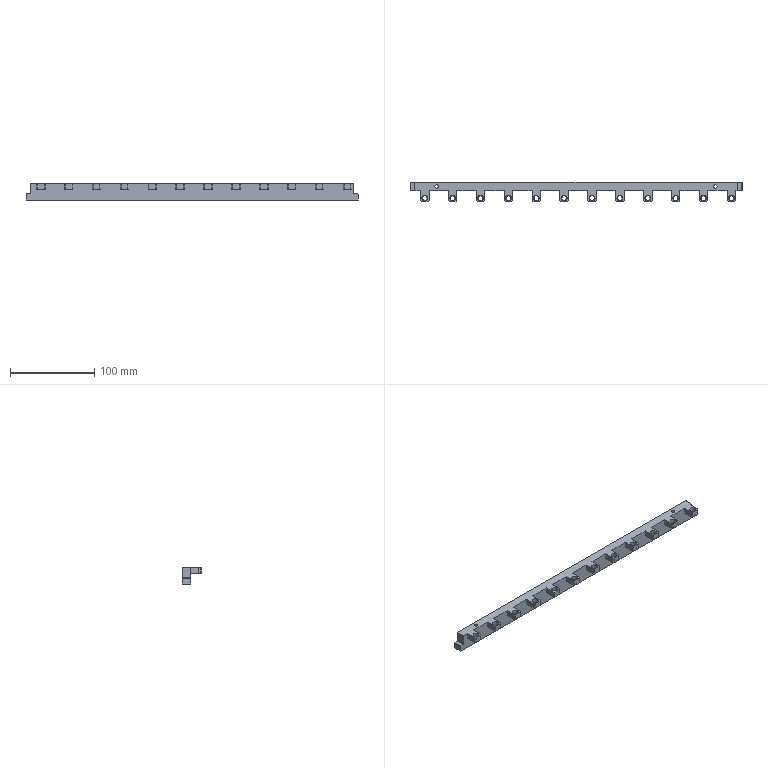Part | NX | features BREP 1 | 1 solid | 180 faces | box 393 x 23 x 20 mm | volume 84586 mm3 | plane 104 | cylinder 68 | cone 8 | commonest cylinder face diameters 5.5 x24 7 x24 2.5 x16 4 x4